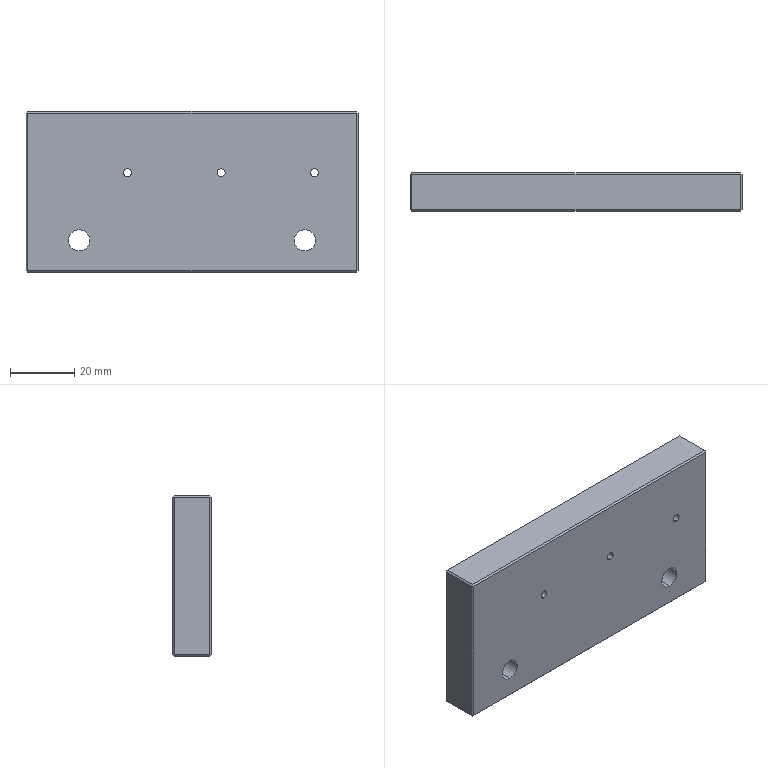Part | STEP file | ND25021-01-JDKM-33-TL | 1 solid | 42 faces | box 103 x 12 x 50 mm | volume 59942 mm3 | plane 28 | cylinder 14 | commonest cylinder face diameters 2.5 x6 6.6 x4 11 x4